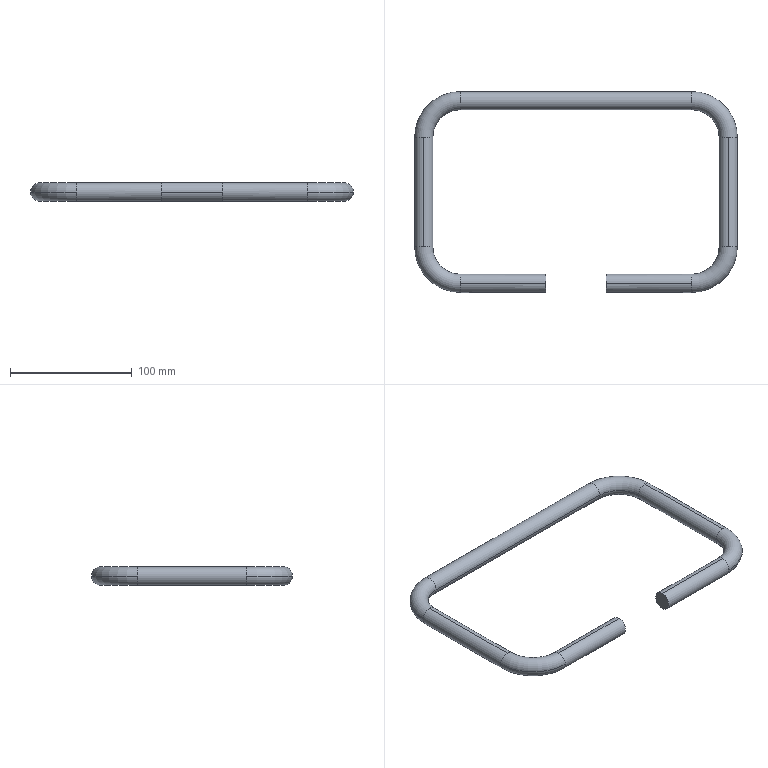Part | SolidWorks | features Sweep 1 | 1 solid | 20 faces | box 265 x 165 x 15 mm | volume 123434 mm3 | cylinder 10 | torus 8 | plane 2 | commonest cylinder face diameters 15 x10
STEP:
#1=CARTESIAN_POINT('',(-150.,30.,7.5));
#2=VERTEX_POINT('',#1);
#3=CARTESIAN_POINT('',(-157.5,30.,0.));
#4=VERTEX_POINT('',#3);
#5=CARTESIAN_POINT('',(-150.,30.,0.));
#6=DIRECTION('',(0.,-1.,0.));
#7=DIRECTION('',(0.,0.,-1.));
#8=AXIS2_PLACEMENT_3D('',#5,#6,#7);
#9=CIRCLE('',#8,7.5);
#10=EDGE_CURVE('',#2,#4,#9,.T.);
#11=ORIENTED_EDGE('',*,*,#10,.T.);
#12=CARTESIAN_POINT('',(-120.,-7.5,0.));
#13=VERTEX_POINT('',#12);
#14=CARTESIAN_POINT('',(-120.,30.,0.));
#15=DIRECTION('',(0.,0.,1.));
#16=DIRECTION('',(1.,0.,0.));
#17=AXIS2_PLACEMENT_3D('',#14,#15,#16);
#18=CIRCLE('',#17,37.5);
#19=EDGE_CURVE('',#4,#13,#18,.T.);
#20=ORIENTED_EDGE('',*,*,#19,.T.);
#21=CARTESIAN_POINT('',(-120.,0.,7.5));
#22=VERTEX_POINT('',#21);
#23=CARTESIAN_POINT('',(-120.,0.,0.));
#24=DIRECTION('',(1.,0.,0.));
#25=DIRECTION('',(0.,0.,-1.));
#26=AXIS2_PLACEMENT_3D('',#23,#24,#25);
#27=CIRCLE('',#26,7.5);
#28=EDGE_CURVE('',#22,#13,#27,.T.);
#29=ORIENTED_EDGE('',*,*,#28,.F.);
#30=CARTESIAN_POINT('',(-120.,7.5,0.));
#31=VERTEX_POINT('',#30);
#32=CARTESIAN_POINT('',(-120.,0.,0.));
#33=DIRECTION('',(1.,0.,0.));
#34=DIRECTION('',(0.,0.,-1.));
#35=AXIS2_PLACEMENT_3D('',#32,#33,#34);
#36=CIRCLE('',#35,7.5);
#37=EDGE_CURVE('',#31,#22,#36,.T.);
#38=ORIENTED_EDGE('',*,*,#37,.F.);
#39=CARTESIAN_POINT('',(-142.5,30.,0.));
#40=VERTEX_POINT('',#39);
#41=CARTESIAN_POINT('',(-120.,30.,0.));
#42=DIRECTION('',(0.,0.,1.));
#43=DIRECTION('',(1.,0.,0.));
#44=AXIS2_PLACEMENT_3D('',#41,#42,#43);
#45=CIRCLE('',#44,22.5);
#46=EDGE_CURVE('',#40,#31,#45,.T.);
#47=ORIENTED_EDGE('',*,*,#46,.F.);
#48=CARTESIAN_POINT('',(-150.,30.,0.));
#49=DIRECTION('',(0.,-1.,0.));
#50=DIRECTION('',(0.,0.,-1.));
#51=AXIS2_PLACEMENT_3D('',#48,#49,#50);
#52=CIRCLE('',#51,7.5);
#53=EDGE_CURVE('',#40,#2,#52,.T.);
#54=ORIENTED_EDGE('',*,*,#53,.T.);
#55=EDGE_LOOP('',(#11,#20,#29,#38,#47,#54));
#56=FACE_OUTER_BOUND('',#55,.T.);
#57=CARTESIAN_POINT('',(-120.,30.,0.));
#58=DIRECTION('',(0.,0.,1.));
#59=DIRECTION('',(1.,0.,0.));
#60=AXIS2_PLACEMENT_3D('',#57,#58,#59);
#61=TOROIDAL_SURFACE('',#60,30.,7.5);
#62=ADVANCED_FACE('',(#56),#61,.T.);
#63=CARTESIAN_POINT('',(-120.,142.5,0.));
#64=VERTEX_POINT('',#63);
#65=CARTESIAN_POINT('',(-120.,157.5,0.));
#66=VERTEX_POINT('',#65);
#67=CARTESIAN_POINT('',(-120.,150.,0.));
#68=DIRECTION('',(-1.,0.,0.));
#69=DIRECTION('',(0.,0.,-1.));
#70=AXIS2_PLACEMENT_3D('',#67,#68,#69);
#71=CIRCLE('',#70,7.5);
#72=EDGE_CURVE('',#64,#66,#71,.T.);
#73=ORIENTED_EDGE('',*,*,#72,.T.);
#74=CARTESIAN_POINT('',(-157.5,120.,0.));
#75=VERTEX_POINT('',#74);
#76=CARTESIAN_POINT('',(-120.,120.,0.));
#77=DIRECTION('',(0.,0.,1.));
#78=DIRECTION('',(1.,0.,0.));
#79=AXIS2_PLACEMENT_3D('',#76,#77,#78);
#80=CIRCLE('',#79,37.5);
#81=EDGE_CURVE('',#66,#75,#80,.T.);
#82=ORIENTED_EDGE('',*,*,#81,.T.);
#83=CARTESIAN_POINT('',(-150.,120.,7.5));
#84=VERTEX_POINT('',#83);
#85=CARTESIAN_POINT('',(-150.,120.,0.));
#86=DIRECTION('',(0.,-1.,0.));
#87=DIRECTION('',(0.,0.,-1.));
#88=AXIS2_PLACEMENT_3D('',#85,#86,#87);
#89=CIRCLE('',#88,7.5);
#90=EDGE_CURVE('',#84,#75,#89,.T.);
#91=ORIENTED_EDGE('',*,*,#90,.F.);
#92=CARTESIAN_POINT('',(-142.5,120.,0.));
#93=VERTEX_POINT('',#92);
#94=CARTESIAN_POINT('',(-150.,120.,0.));
#95=DIRECTION('',(0.,-1.,0.));
#96=DIRECTION('',(0.,0.,-1.));
#97=AXIS2_PLACEMENT_3D('',#94,#95,#96);
#98=CIRCLE('',#97,7.5);
#99=EDGE_CURVE('',#93,#84,#98,.T.);
#100=ORIENTED_EDGE('',*,*,#99,.F.);
#101=CARTESIAN_POINT('',(-120.,120.,0.));
#102=DIRECTION('',(0.,0.,1.));
#103=DIRECTION('',(1.,0.,0.));
#104=AXIS2_PLACEMENT_3D('',#101,#102,#103);
#105=CIRCLE('',#104,22.5);
#106=EDGE_CURVE('',#64,#93,#105,.T.);
#107=ORIENTED_EDGE('',*,*,#106,.F.);
#108=EDGE_LOOP('',(#73,#82,#91,#100,#107));
#109=FACE_OUTER_BOUND('',#108,.T.);
#110=CARTESIAN_POINT('',(-120.,120.,0.));
#111=DIRECTION('',(0.,0.,1.));
#112=DIRECTION('',(1.,0.,0.));
#113=AXIS2_PLACEMENT_3D('',#110,#111,#112);
#114=TOROIDAL_SURFACE('',#113,30.,7.5);
#115=ADVANCED_FACE('',(#109),#114,.T.);
#116=CARTESIAN_POINT('',(100.,120.,7.5));
#117=VERTEX_POINT('',#116);
#118=CARTESIAN_POINT('',(107.5,120.,0.));
#119=VERTEX_POINT('',#118);
#120=CARTESIAN_POINT('',(100.,120.,0.));
#121=DIRECTION('',(0.,1.,0.));
#122=DIRECTION('',(0.,0.,-1.));
#123=AXIS2_PLACEMENT_3D('',#120,#121,#122);
#124=CIRCLE('',#123,7.5);
#125=EDGE_CURVE('',#117,#119,#124,.T.);
#126=ORIENTED_EDGE('',*,*,#125,.T.);
#127=CARTESIAN_POINT('',(70.,157.5,0.));
#128=VERTEX_POINT('',#127);
#129=CARTESIAN_POINT('',(70.,120.,0.));
#130=DIRECTION('',(0.,0.,1.));
#131=DIRECTION('',(1.,0.,0.));
#132=AXIS2_PLACEMENT_3D('',#129,#130,#131);
#133=CIRCLE('',#132,37.5);
#134=EDGE_CURVE('',#119,#128,#133,.T.);
#135=ORIENTED_EDGE('',*,*,#134,.T.);
#136=CARTESIAN_POINT('',(70.,142.5,0.));
#137=VERTEX_POINT('',#136);
#138=CARTESIAN_POINT('',(70.,150.,0.));
#139=DIRECTION('',(-1.,0.,0.));
#140=DIRECTION('',(0.,0.,-1.));
#141=AXIS2_PLACEMENT_3D('',#138,#139,#140);
#142=CIRCLE('',#141,7.5);
#143=EDGE_CURVE('',#137,#128,#142,.T.);
#144=ORIENTED_EDGE('',*,*,#143,.F.);
#145=CARTESIAN_POINT('',(92.5,120.,0.));
#146=VERTEX_POINT('',#145);
#147=CARTESIAN_POINT('',(70.,120.,0.));
#148=DIRECTION('',(0.,0.,1.));
#149=DIRECTION('',(1.,0.,0.));
#150=AXIS2_PLACEMENT_3D('',#147,#148,#149);
#151=CIRCLE('',#150,22.5);
#152=EDGE_CURVE('',#146,#137,#151,.T.);
#153=ORIENTED_EDGE('',*,*,#152,.F.);
#154=CARTESIAN_POINT('',(100.,120.,0.));
#155=DIRECTION('',(0.,1.,0.));
#156=DIRECTION('',(0.,0.,-1.));
#157=AXIS2_PLACEMENT_3D('',#154,#155,#156);
#158=CIRCLE('',#157,7.5);
#159=EDGE_CURVE('',#146,#117,#158,.T.);
#160=ORIENTED_EDGE('',*,*,#159,.T.);
#161=EDGE_LOOP('',(#126,#135,#144,#153,#160));
#162=FACE_OUTER_BOUND('',#161,.T.);
#163=CARTESIAN_POINT('',(70.,120.,0.));
#164=DIRECTION('',(0.,0.,1.));
#165=DIRECTION('',(1.,0.,0.));
#166=AXIS2_PLACEMENT_3D('',#163,#164,#165);
#167=TOROIDAL_SURFACE('',#166,30.,7.5);
#168=ADVANCED_FACE('',(#162),#167,.T.);
#169=CARTESIAN_POINT('',(70.,0.,7.5));
#170=VERTEX_POINT('',#169);
#171=CARTESIAN_POINT('',(70.,-7.5,0.));
#172=VERTEX_POINT('',#171);
#173=CARTESIAN_POINT('',(70.,0.,0.));
#174=DIRECTION('',(1.,0.,0.));
#175=DIRECTION('',(0.,0.,-1.));
#176=AXIS2_PLACEMENT_3D('',#173,#174,#175);
#177=CIRCLE('',#176,7.5);
#178=EDGE_CURVE('',#170,#172,#177,.T.);
#179=ORIENTED_EDGE('',*,*,#178,.T.);
#180=CARTESIAN_POINT('',(107.5,30.,0.));
#181=VERTEX_POINT('',#180);
#182=CARTESIAN_POINT('',(70.,30.,0.));
#183=DIRECTION('',(0.,0.,1.));
#184=DIRECTION('',(1.,0.,0.));
#185=AXIS2_PLACEMENT_3D('',#182,#183,#184);
#186=CIRCLE('',#185,37.5);
#187=EDGE_CURVE('',#172,#181,#186,.T.);
#188=ORIENTED_EDGE('',*,*,#187,.T.);
#189=CARTESIAN_POINT('',(100.,30.,7.5));
#190=VERTEX_POINT('',#189);
#191=CARTESIAN_POINT('',(100.,30.,0.));
#192=DIRECTION('',(0.,1.,0.));
#193=DIRECTION('',(0.,0.,-1.));
#194=AXIS2_PLACEMENT_3D('',#191,#192,#193);
#195=CIRCLE('',#194,7.5);
#196=EDGE_CURVE('',#190,#181,#195,.T.);
#197=ORIENTED_EDGE('',*,*,#196,.F.);
#198=CARTESIAN_POINT('',(92.5,30.,0.));
#199=VERTEX_POINT('',#198);
#200=CARTESIAN_POINT('',(100.,30.,0.));
#201=DIRECTION('',(0.,1.,0.));
#202=DIRECTION('',(0.,0.,-1.));
#203=AXIS2_PLACEMENT_3D('',#200,#201,#202);
#204=CIRCLE('',#203,7.5);
#205=EDGE_CURVE('',#199,#190,#204,.T.);
#206=ORIENTED_EDGE('',*,*,#205,.F.);
#207=CARTESIAN_POINT('',(70.,7.5,0.));
#208=VERTEX_POINT('',#207);
#209=CARTESIAN_POINT('',(70.,30.,0.));
#210=DIRECTION('',(0.,0.,1.));
#211=DIRECTION('',(1.,0.,0.));
#212=AXIS2_PLACEMENT_3D('',#209,#210,#211);
#213=CIRCLE('',#212,22.5);
#214=EDGE_CURVE('',#208,#199,#213,.T.);
#215=ORIENTED_EDGE('',*,*,#214,.F.);
#216=CARTESIAN_POINT('',(70.,0.,0.));
#217=DIRECTION('',(1.,0.,0.));
#218=DIRECTION('',(0.,0.,-1.));
#219=AXIS2_PLACEMENT_3D('',#216,#217,#218);
#220=CIRCLE('',#219,7.5);
#221=EDGE_CURVE('',#208,#170,#220,.T.);
#222=ORIENTED_EDGE('',*,*,#221,.T.);
#223=EDGE_LOOP('',(#179,#188,#197,#206,#215,#222));
#224=FACE_OUTER_BOUND('',#223,.T.);
#225=CARTESIAN_POINT('',(70.,30.,0.));
#226=DIRECTION('',(0.,0.,1.));
#227=DIRECTION('',(1.,0.,0.));
#228=AXIS2_PLACEMENT_3D('',#225,#226,#227);
#229=TOROIDAL_SURFACE('',#228,30.,7.5);
#230=ADVANCED_FACE('',(#224),#229,.T.);
#231=CARTESIAN_POINT('',(-120.,0.,-7.5));
#232=VERTEX_POINT('',#231);
#233=CARTESIAN_POINT('',(-120.,0.,0.));
#234=DIRECTION('',(1.,0.,0.));
#235=DIRECTION('',(0.,0.,-1.));
#236=AXIS2_PLACEMENT_3D('',#233,#234,#235);
#237=CIRCLE('',#236,7.5);
#238=EDGE_CURVE('',#232,#31,#237,.T.);
#239=ORIENTED_EDGE('',*,*,#238,.T.);
#240=ORIENTED_EDGE('',*,*,#37,.T.);
#241=CARTESIAN_POINT('',(-50.,0.,7.5));
#242=VERTEX_POINT('',#241);
#243=CARTESIAN_POINT('',(-120.,0.,7.5));
#244=DIRECTION('',(1.,0.,0.));
#245=VECTOR('',#244,1000.);
#246=LINE('',#243,#245);
#247=EDGE_CURVE('',#22,#242,#246,.T.);
#248=ORIENTED_EDGE('',*,*,#247,.T.);
#249=CARTESIAN_POINT('',(-50.,0.,-7.5));
#250=VERTEX_POINT('',#249);
#251=CARTESIAN_POINT('',(-50.,0.,0.));
#252=DIRECTION('',(1.,0.,0.));
#253=DIRECTION('',(0.,0.,-1.));
#254=AXIS2_PLACEMENT_3D('',#251,#252,#253);
#255=CIRCLE('',#254,7.5);
#256=EDGE_CURVE('',#250,#242,#255,.T.);
#257=ORIENTED_EDGE('',*,*,#256,.F.);
#258=CARTESIAN_POINT('',(-120.,0.,-7.5));
#259=DIRECTION('',(1.,0.,0.));
#260=VECTOR('',#259,1000.);
#261=LINE('',#258,#260);
#262=EDGE_CURVE('',#232,#250,#261,.T.);
#263=ORIENTED_EDGE('',*,*,#262,.F.);
#264=EDGE_LOOP('',(#239,#240,#248,#257,#263));
#265=FACE_OUTER_BOUND('',#264,.T.);
#266=CARTESIAN_POINT('',(-120.,0.,0.));
#267=DIRECTION('',(1.,0.,0.));
#268=DIRECTION('',(0.,0.,-1.));
#269=AXIS2_PLACEMENT_3D('',#266,#267,#268);
#270=CYLINDRICAL_SURFACE('',#269,7.5);
#271=ADVANCED_FACE('',(#265),#270,.T.);
#272=CARTESIAN_POINT('',(-150.,120.,-7.5));
#273=VERTEX_POINT('',#272);
#274=CARTESIAN_POINT('',(-150.,120.,0.));
#275=DIRECTION('',(0.,-1.,0.));
#276=DIRECTION('',(0.,0.,-1.));
#277=AXIS2_PLACEMENT_3D('',#274,#275,#276);
#278=CIRCLE('',#277,7.5);
#279=EDGE_CURVE('',#273,#93,#278,.T.);
#280=ORIENTED_EDGE('',*,*,#279,.T.);
#281=ORIENTED_EDGE('',*,*,#99,.T.);
#282=CARTESIAN_POINT('',(-150.,120.,7.5));
#283=DIRECTION('',(0.,-1.,0.));
#284=VECTOR('',#283,1000.);
#285=LINE('',#282,#284);
#286=EDGE_CURVE('',#84,#2,#285,.T.);
#287=ORIENTED_EDGE('',*,*,#286,.T.);
#288=ORIENTED_EDGE('',*,*,#53,.F.);
#289=CARTESIAN_POINT('',(-150.,30.,-7.5));
#290=VERTEX_POINT('',#289);
#291=CARTESIAN_POINT('',(-150.,30.,0.));
#292=DIRECTION('',(0.,-1.,0.));
#293=DIRECTION('',(0.,0.,-1.));
#294=AXIS2_PLACEMENT_3D('',#291,#292,#293);
#295=CIRCLE('',#294,7.5);
#296=EDGE_CURVE('',#290,#40,#295,.T.);
#297=ORIENTED_EDGE('',*,*,#296,.F.);
#298=CARTESIAN_POINT('',(-150.,120.,-7.5));
#299=DIRECTION('',(0.,-1.,0.));
#300=VECTOR('',#299,1000.);
#301=LINE('',#298,#300);
#302=EDGE_CURVE('',#273,#290,#301,.T.);
#303=ORIENTED_EDGE('',*,*,#302,.F.);
#304=EDGE_LOOP('',(#280,#281,#287,#288,#297,#303));
#305=FACE_OUTER_BOUND('',#304,.T.);
#306=CARTESIAN_POINT('',(-150.,120.,0.));
#307=DIRECTION('',(0.,-1.,0.));
#308=DIRECTION('',(0.,0.,-1.));
#309=AXIS2_PLACEMENT_3D('',#306,#307,#308);
#310=CYLINDRICAL_SURFACE('',#309,7.5);
#311=ADVANCED_FACE('',(#305),#310,.T.);
#312=ORIENTED_EDGE('',*,*,#143,.T.);
#313=CARTESIAN_POINT('',(70.,157.5,0.));
#314=DIRECTION('',(-1.,0.,0.));
#315=VECTOR('',#314,1000.);
#316=LINE('',#313,#315);
#317=EDGE_CURVE('',#128,#66,#316,.T.);
#318=ORIENTED_EDGE('',*,*,#317,.T.);
#319=ORIENTED_EDGE('',*,*,#72,.F.);
#320=CARTESIAN_POINT('',(70.,142.5,0.));
#321=DIRECTION('',(-1.,0.,0.));
#322=VECTOR('',#321,1000.);
#323=LINE('',#320,#322);
#324=EDGE_CURVE('',#137,#64,#323,.T.);
#325=ORIENTED_EDGE('',*,*,#324,.F.);
#326=EDGE_LOOP('',(#312,#318,#319,#325));
#327=FACE_OUTER_BOUND('',#326,.T.);
#328=CARTESIAN_POINT('',(70.,150.,0.));
#329=DIRECTION('',(-1.,0.,0.));
#330=DIRECTION('',(0.,-1.,0.));
#331=AXIS2_PLACEMENT_3D('',#328,#329,#330);
#332=CYLINDRICAL_SURFACE('',#331,7.5);
#333=ADVANCED_FACE('',(#327),#332,.T.);
#334=ORIENTED_EDGE('',*,*,#196,.T.);
#335=CARTESIAN_POINT('',(100.,30.,-7.5));
#336=VERTEX_POINT('',#335);
#337=CARTESIAN_POINT('',(100.,30.,0.));
#338=DIRECTION('',(0.,1.,0.));
#339=DIRECTION('',(0.,0.,-1.));
#340=AXIS2_PLACEMENT_3D('',#337,#338,#339);
#341=CIRCLE('',#340,7.5);
#342=EDGE_CURVE('',#181,#336,#341,.T.);
#343=ORIENTED_EDGE('',*,*,#342,.T.);
#344=CARTESIAN_POINT('',(100.,120.,-7.5));
#345=VERTEX_POINT('',#344);
#346=CARTESIAN_POINT('',(100.,30.,-7.5));
#347=DIRECTION('',(0.,1.,0.));
#348=VECTOR('',#347,1000.);
#349=LINE('',#346,#348);
#350=EDGE_CURVE('',#336,#345,#349,.T.);
#351=ORIENTED_EDGE('',*,*,#350,.T.);
#352=CARTESIAN_POINT('',(100.,120.,0.));
#353=DIRECTION('',(0.,1.,0.));
#354=DIRECTION('',(0.,0.,-1.));
#355=AXIS2_PLACEMENT_3D('',#352,#353,#354);
#356=CIRCLE('',#355,7.5);
#357=EDGE_CURVE('',#119,#345,#356,.T.);
#358=ORIENTED_EDGE('',*,*,#357,.F.);
#359=ORIENTED_EDGE('',*,*,#125,.F.);
#360=CARTESIAN_POINT('',(100.,30.,7.5));
#361=DIRECTION('',(0.,1.,0.));
#362=VECTOR('',#361,1000.);
#363=LINE('',#360,#362);
#364=EDGE_CURVE('',#190,#117,#363,.T.);
#365=ORIENTED_EDGE('',*,*,#364,.F.);
#366=EDGE_LOOP('',(#334,#343,#351,#358,#359,#365));
#367=FACE_OUTER_BOUND('',#366,.T.);
#368=CARTESIAN_POINT('',(100.,30.,0.));
#369=DIRECTION('',(0.,1.,0.));
#370=DIRECTION('',(0.,0.,1.));
#371=AXIS2_PLACEMENT_3D('',#368,#369,#370);
#372=CYLINDRICAL_SURFACE('',#371,7.5);
#373=ADVANCED_FACE('',(#367),#372,.T.);
#374=CARTESIAN_POINT('',(0.,0.,-7.5));
#375=VERTEX_POINT('',#374);
#376=CARTESIAN_POINT('',(0.,0.,7.5));
#377=VERTEX_POINT('',#376);
#378=CARTESIAN_POINT('',(0.,0.,0.));
#379=DIRECTION('',(1.,0.,0.));
#380=DIRECTION('',(0.,0.,-1.));
#381=AXIS2_PLACEMENT_3D('',#378,#379,#380);
#382=CIRCLE('',#381,7.5);
#383=EDGE_CURVE('',#375,#377,#382,.T.);
#384=ORIENTED_EDGE('',*,*,#383,.T.);
#385=CARTESIAN_POINT('',(0.,0.,7.5));
#386=DIRECTION('',(1.,0.,0.));
#387=VECTOR('',#386,1000.);
#388=LINE('',#385,#387);
#389=EDGE_CURVE('',#377,#170,#388,.T.);
#390=ORIENTED_EDGE('',*,*,#389,.T.);
#391=ORIENTED_EDGE('',*,*,#221,.F.);
#392=CARTESIAN_POINT('',(70.,0.,-7.5));
#393=VERTEX_POINT('',#392);
#394=CARTESIAN_POINT('',(70.,0.,0.));
#395=DIRECTION('',(1.,0.,0.));
#396=DIRECTION('',(0.,0.,-1.));
#397=AXIS2_PLACEMENT_3D('',#394,#395,#396);
#398=CIRCLE('',#397,7.5);
#399=EDGE_CURVE('',#393,#208,#398,.T.);
#400=ORIENTED_EDGE('',*,*,#399,.F.);
#401=CARTESIAN_POINT('',(0.,0.,-7.5));
#402=DIRECTION('',(1.,0.,0.));
#403=VECTOR('',#402,1000.);
#404=LINE('',#401,#403);
#405=EDGE_CURVE('',#375,#393,#404,.T.);
#406=ORIENTED_EDGE('',*,*,#405,.F.);
#407=EDGE_LOOP('',(#384,#390,#391,#400,#406));
#408=FACE_OUTER_BOUND('',#407,.T.);
#409=CARTESIAN_POINT('',(0.,0.,0.));
#410=DIRECTION('',(1.,0.,0.));
#411=DIRECTION('',(0.,0.,-1.));
#412=AXIS2_PLACEMENT_3D('',#409,#410,#411);
#413=CYLINDRICAL_SURFACE('',#412,7.5);
#414=ADVANCED_FACE('',(#408),#413,.T.);
#415=ORIENTED_EDGE('',*,*,#247,.F.);
#416=ORIENTED_EDGE('',*,*,#28,.T.);
#417=CARTESIAN_POINT('',(-120.,0.,0.));
#418=DIRECTION('',(1.,0.,0.));
#419=DIRECTION('',(0.,0.,-1.));
#420=AXIS2_PLACEMENT_3D('',#417,#418,#419);
#421=CIRCLE('',#420,7.5);
#422=EDGE_CURVE('',#13,#232,#421,.T.);
#423=ORIENTED_EDGE('',*,*,#422,.T.);
#424=ORIENTED_EDGE('',*,*,#262,.T.);
#425=CARTESIAN_POINT('',(-50.,0.,0.));
#426=DIRECTION('',(1.,0.,0.));
#427=DIRECTION('',(0.,0.,-1.));
#428=AXIS2_PLACEMENT_3D('',#425,#426,#427);
#429=CIRCLE('',#428,7.5);
#430=EDGE_CURVE('',#242,#250,#429,.T.);
#431=ORIENTED_EDGE('',*,*,#430,.F.);
#432=EDGE_LOOP('',(#415,#416,#423,#424,#431));
#433=FACE_OUTER_BOUND('',#432,.T.);
#434=CARTESIAN_POINT('',(-120.,0.,0.));
#435=DIRECTION('',(1.,0.,0.));
#436=DIRECTION('',(0.,0.,-1.));
#437=AXIS2_PLACEMENT_3D('',#434,#435,#436);
#438=CYLINDRICAL_SURFACE('',#437,7.5);
#439=ADVANCED_FACE('',(#433),#438,.T.);
#440=ORIENTED_EDGE('',*,*,#19,.F.);
#441=CARTESIAN_POINT('',(-150.,30.,0.));
#442=DIRECTION('',(0.,-1.,0.));
#443=DIRECTION('',(0.,0.,-1.));
#444=AXIS2_PLACEMENT_3D('',#441,#442,#443);
#445=CIRCLE('',#444,7.5);
#446=EDGE_CURVE('',#4,#290,#445,.T.);
#447=ORIENTED_EDGE('',*,*,#446,.T.);
#448=ORIENTED_EDGE('',*,*,#296,.T.);
#449=ORIENTED_EDGE('',*,*,#46,.T.);
#450=ORIENTED_EDGE('',*,*,#238,.F.);
#451=ORIENTED_EDGE('',*,*,#422,.F.);
#452=EDGE_LOOP('',(#440,#447,#448,#449,#450,#451));
#453=FACE_OUTER_BOUND('',#452,.T.);
#454=CARTESIAN_POINT('',(-120.,30.,0.));
#455=DIRECTION('',(0.,0.,1.));
#456=DIRECTION('',(1.,0.,0.));
#457=AXIS2_PLACEMENT_3D('',#454,#455,#456);
#458=TOROIDAL_SURFACE('',#457,30.,7.5);
#459=ADVANCED_FACE('',(#453),#458,.T.);
#460=ORIENTED_EDGE('',*,*,#286,.F.);
#461=ORIENTED_EDGE('',*,*,#90,.T.);
#462=CARTESIAN_POINT('',(-150.,120.,0.));
#463=DIRECTION('',(0.,-1.,0.));
#464=DIRECTION('',(0.,0.,-1.));
#465=AXIS2_PLACEMENT_3D('',#462,#463,#464);
#466=CIRCLE('',#465,7.5);
#467=EDGE_CURVE('',#75,#273,#466,.T.);
#468=ORIENTED_EDGE('',*,*,#467,.T.);
#469=ORIENTED_EDGE('',*,*,#302,.T.);
#470=ORIENTED_EDGE('',*,*,#446,.F.);
#471=ORIENTED_EDGE('',*,*,#10,.F.);
#472=EDGE_LOOP('',(#460,#461,#468,#469,#470,#471));
#473=FACE_OUTER_BOUND('',#472,.T.);
#474=CARTESIAN_POINT('',(-150.,120.,0.));
#475=DIRECTION('',(0.,-1.,0.));
#476=DIRECTION('',(0.,0.,-1.));
#477=AXIS2_PLACEMENT_3D('',#474,#475,#476);
#478=CYLINDRICAL_SURFACE('',#477,7.5);
#479=ADVANCED_FACE('',(#473),#478,.T.);
#480=ORIENTED_EDGE('',*,*,#81,.F.);
#481=CARTESIAN_POINT('',(-120.,150.,0.));
#482=DIRECTION('',(-1.,0.,0.));
#483=DIRECTION('',(0.,0.,-1.));
#484=AXIS2_PLACEMENT_3D('',#481,#482,#483);
#485=CIRCLE('',#484,7.5);
#486=EDGE_CURVE('',#66,#64,#485,.T.);
#487=ORIENTED_EDGE('',*,*,#486,.T.);
#488=ORIENTED_EDGE('',*,*,#106,.T.);
#489=ORIENTED_EDGE('',*,*,#279,.F.);
#490=ORIENTED_EDGE('',*,*,#467,.F.);
#491=EDGE_LOOP('',(#480,#487,#488,#489,#490));
#492=FACE_OUTER_BOUND('',#491,.T.);
#493=CARTESIAN_POINT('',(-120.,120.,0.));
#494=DIRECTION('',(0.,0.,1.));
#495=DIRECTION('',(1.,0.,0.));
#496=AXIS2_PLACEMENT_3D('',#493,#494,#495);
#497=TOROIDAL_SURFACE('',#496,30.,7.5);
#498=ADVANCED_FACE('',(#492),#497,.T.);
#499=ORIENTED_EDGE('',*,*,#317,.F.);
#500=CARTESIAN_POINT('',(70.,150.,0.));
#501=DIRECTION('',(-1.,0.,0.));
#502=DIRECTION('',(0.,0.,-1.));
#503=AXIS2_PLACEMENT_3D('',#500,#501,#502);
#504=CIRCLE('',#503,7.5);
#505=EDGE_CURVE('',#128,#137,#504,.T.);
#506=ORIENTED_EDGE('',*,*,#505,.T.);
#507=ORIENTED_EDGE('',*,*,#324,.T.);
#508=ORIENTED_EDGE('',*,*,#486,.F.);
#509=EDGE_LOOP('',(#499,#506,#507,#508));
#510=FACE_OUTER_BOUND('',#509,.T.);
#511=CARTESIAN_POINT('',(70.,150.,0.));
#512=DIRECTION('',(-1.,0.,0.));
#513=DIRECTION('',(0.,-1.,0.));
#514=AXIS2_PLACEMENT_3D('',#511,#512,#513);
#515=CYLINDRICAL_SURFACE('',#514,7.5);
#516=ADVANCED_FACE('',(#510),#515,.T.);
#517=ORIENTED_EDGE('',*,*,#134,.F.);
#518=ORIENTED_EDGE('',*,*,#357,.T.);
#519=CARTESIAN_POINT('',(100.,120.,0.));
#520=DIRECTION('',(0.,1.,0.));
#521=DIRECTION('',(0.,0.,-1.));
#522=AXIS2_PLACEMENT_3D('',#519,#520,#521);
#523=CIRCLE('',#522,7.5);
#524=EDGE_CURVE('',#345,#146,#523,.T.);
#525=ORIENTED_EDGE('',*,*,#524,.T.);
#526=ORIENTED_EDGE('',*,*,#152,.T.);
#527=ORIENTED_EDGE('',*,*,#505,.F.);
#528=EDGE_LOOP('',(#517,#518,#525,#526,#527));
#529=FACE_OUTER_BOUND('',#528,.T.);
#530=CARTESIAN_POINT('',(70.,120.,0.));
#531=DIRECTION('',(0.,0.,1.));
#532=DIRECTION('',(1.,0.,0.));
#533=AXIS2_PLACEMENT_3D('',#530,#531,#532);
#534=TOROIDAL_SURFACE('',#533,30.,7.5);
#535=ADVANCED_FACE('',(#529),#534,.T.);
#536=ORIENTED_EDGE('',*,*,#350,.F.);
#537=CARTESIAN_POINT('',(100.,30.,0.));
#538=DIRECTION('',(0.,1.,0.));
#539=DIRECTION('',(0.,0.,-1.));
#540=AXIS2_PLACEMENT_3D('',#537,#538,#539);
#541=CIRCLE('',#540,7.5);
#542=EDGE_CURVE('',#336,#199,#541,.T.);
#543=ORIENTED_EDGE('',*,*,#542,.T.);
#544=ORIENTED_EDGE('',*,*,#205,.T.);
#545=ORIENTED_EDGE('',*,*,#364,.T.);
#546=ORIENTED_EDGE('',*,*,#159,.F.);
#547=ORIENTED_EDGE('',*,*,#524,.F.);
#548=EDGE_LOOP('',(#536,#543,#544,#545,#546,#547));
#549=FACE_OUTER_BOUND('',#548,.T.);
#550=CARTESIAN_POINT('',(100.,30.,0.));
#551=DIRECTION('',(0.,1.,0.));
#552=DIRECTION('',(0.,0.,1.));
#553=AXIS2_PLACEMENT_3D('',#550,#551,#552);
#554=CYLINDRICAL_SURFACE('',#553,7.5);
#555=ADVANCED_FACE('',(#549),#554,.T.);
#556=ORIENTED_EDGE('',*,*,#187,.F.);
#557=CARTESIAN_POINT('',(70.,0.,0.));
#558=DIRECTION('',(1.,0.,0.));
#559=DIRECTION('',(0.,0.,-1.));
#560=AXIS2_PLACEMENT_3D('',#557,#558,#559);
#561=CIRCLE('',#560,7.5);
#562=EDGE_CURVE('',#172,#393,#561,.T.);
#563=ORIENTED_EDGE('',*,*,#562,.T.);
#564=ORIENTED_EDGE('',*,*,#399,.T.);
#565=ORIENTED_EDGE('',*,*,#214,.T.);
#566=ORIENTED_EDGE('',*,*,#542,.F.);
#567=ORIENTED_EDGE('',*,*,#342,.F.);
#568=EDGE_LOOP('',(#556,#563,#564,#565,#566,#567));
#569=FACE_OUTER_BOUND('',#568,.T.);
#570=CARTESIAN_POINT('',(70.,30.,0.));
#571=DIRECTION('',(0.,0.,1.));
#572=DIRECTION('',(1.,0.,0.));
#573=AXIS2_PLACEMENT_3D('',#570,#571,#572);
#574=TOROIDAL_SURFACE('',#573,30.,7.5);
#575=ADVANCED_FACE('',(#569),#574,.T.);
#576=ORIENTED_EDGE('',*,*,#389,.F.);
#577=CARTESIAN_POINT('',(0.,0.,0.));
#578=DIRECTION('',(1.,0.,0.));
#579=DIRECTION('',(0.,0.,-1.));
#580=AXIS2_PLACEMENT_3D('',#577,#578,#579);
#581=CIRCLE('',#580,7.5);
#582=EDGE_CURVE('',#377,#375,#581,.T.);
#583=ORIENTED_EDGE('',*,*,#582,.T.);
#584=ORIENTED_EDGE('',*,*,#405,.T.);
#585=ORIENTED_EDGE('',*,*,#562,.F.);
#586=ORIENTED_EDGE('',*,*,#178,.F.);
#587=EDGE_LOOP('',(#576,#583,#584,#585,#586));
#588=FACE_OUTER_BOUND('',#587,.T.);
#589=CARTESIAN_POINT('',(0.,0.,0.));
#590=DIRECTION('',(1.,0.,0.));
#591=DIRECTION('',(0.,0.,-1.));
#592=AXIS2_PLACEMENT_3D('',#589,#590,#591);
#593=CYLINDRICAL_SURFACE('',#592,7.5);
#594=ADVANCED_FACE('',(#588),#593,.T.);
#595=ORIENTED_EDGE('',*,*,#256,.T.);
#596=ORIENTED_EDGE('',*,*,#430,.T.);
#597=EDGE_LOOP('',(#595,#596));
#598=FACE_OUTER_BOUND('',#597,.T.);
#599=CARTESIAN_POINT('',(-50.,0.,0.));
#600=DIRECTION('',(1.,0.,0.));
#601=DIRECTION('',(0.,0.,-1.));
#602=AXIS2_PLACEMENT_3D('',#599,#600,#601);
#603=PLANE('',#602);
#604=ADVANCED_FACE('',(#598),#603,.T.);
#605=ORIENTED_EDGE('',*,*,#383,.F.);
#606=ORIENTED_EDGE('',*,*,#582,.F.);
#607=EDGE_LOOP('',(#605,#606));
#608=FACE_OUTER_BOUND('',#607,.T.);
#609=CARTESIAN_POINT('',(0.,0.,0.));
#610=DIRECTION('',(1.,0.,0.));
#611=DIRECTION('',(0.,0.,-1.));
#612=AXIS2_PLACEMENT_3D('',#609,#610,#611);
#613=PLANE('',#612);
#614=ADVANCED_FACE('',(#608),#613,.F.);
#615=CLOSED_SHELL('',(#62,#115,#168,#230,#271,#311,#333,#373,#414,#439,#459,#479,#498,#516,#535,#555,#575,#594,#604,#614));
#616=MANIFOLD_SOLID_BREP('',#615);
#617=CARTESIAN_POINT('',(0.,0.,0.));
#618=DIRECTION('',(0.,0.,1.));
#619=DIRECTION('',(1.,0.,0.));
#620=AXIS2_PLACEMENT_3D('',#617,#618,#619);
#621=(LENGTH_UNIT()NAMED_UNIT(*)SI_UNIT(.MILLI.,.METRE.));
#622=UNCERTAINTY_MEASURE_WITH_UNIT(LENGTH_MEASURE(0.00001),#621,'','');
#623=(NAMED_UNIT(*)PLANE_ANGLE_UNIT()SI_UNIT($,.RADIAN.));
#624=(NAMED_UNIT(*)SI_UNIT($,.STERADIAN.)SOLID_ANGLE_UNIT());
#625=(GEOMETRIC_REPRESENTATION_CONTEXT(3)GLOBAL_UNCERTAINTY_ASSIGNED_CONTEXT((#622))GLOBAL_UNIT_ASSIGNED_CONTEXT((#621,#623,#624))REPRESENTATION_CONTEXT('',''));
#626=ADVANCED_BREP_SHAPE_REPRESENTATION('',(#616,#620),#625);